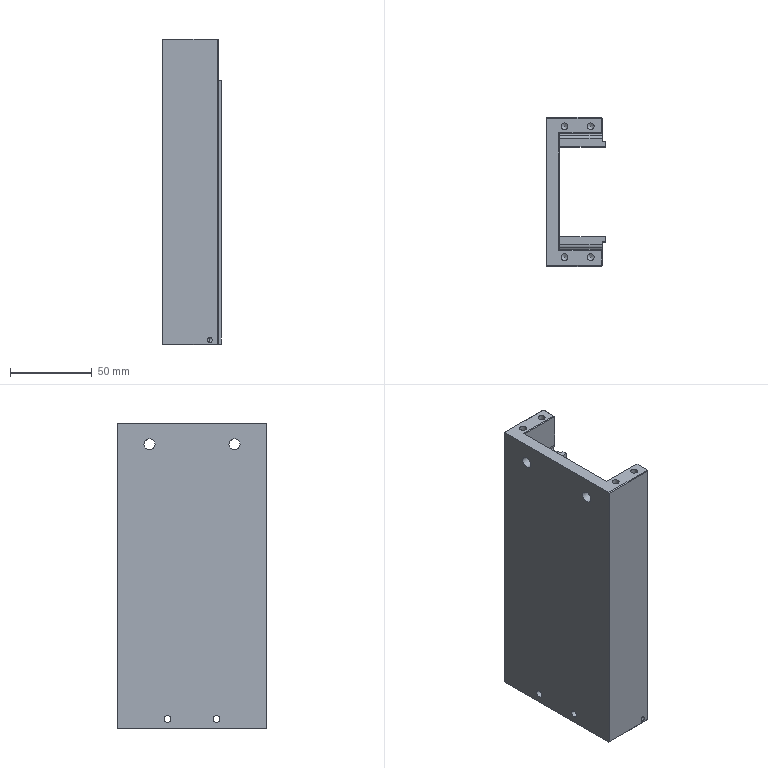CAM job | NX | 3+2 milling, drilling | part box 36 x 91 x 187 mm | stock box 40 x 100 x 192 mm
Tools:
number,name,description,diameter,corner_radius,flute_length,length,flutes
18,D2,平底铣刀-粗,2.0,0.0,50.0,75.0,2
9,D10,平底铣刀-粗,10.0,0.0,35.0,75.0,2
19,D2-J,平底铣刀-精,2.0,0.0,50.0,75.0,2
11,D3-J,平底铣刀-精,2.95,0.0,50.0,75.0,2
7,D6-J,平底铣刀-精,6.0,0.0,25.0,75.0,2
10,D10-J,平底铣刀-精,10.0,0.0,35.0,75.0,2
1,D80R0.8飞刀,圆鼻刀-粗,80.0,0.8,50.0,75.0,2
1,D80R0.8飞刀-J,圆鼻刀-精,80.0,0.8,50.0,75.0,2
2,D6倒角刀,倒角刀,6.0,0.0,3.0,25.0,2
20,M3X0.5,丝锥,2.5,0.0,35.0,50.0,2
22,M5X0.8,丝锥,4.2,0.0,35.0,50.0,2
23,M8X1.25,丝锥,6.8,0.0,35.0,50.0,2
12,ZT2.5,钻头,2.5,0.0,35.0,50.0,2
17,ZT2.8,钻头,2.8,0.0,35.0,50.0,2
16,ZT6.8,钻头,6.8,0.0,35.0,50.0,2
14,DRILL4.2,Twist Drill 4.2 mm,4.2,0.0,41.0,41.738,2
Operations:
program,operation,operation_type,tool,method,geometry_group,spindle_rpm,surface_speed,feed_per_tooth,feed_cut,feed_plunge,cut_length_mm,path_length_mm,cut_time_min,machine_time_min
B,FLOORMILL_FACEROUGH_COPY,VolumeBased25DMillingOperation,D80R0.8飞刀,LAYERROUGH-DEPTHK-STEPG,W-B,2800.0,703.696,0.5357,3000.0,100.0,4141.882,4389.788,1.381,1.405
B,FLOORMILL_FACEFINISH_COPY,VolumeBased25DMillingOperation,D80R0.8飞刀-J,SIDEFINISH-DEPTHK-STEPG,W-B,4000.0,1005.28,0.125,1000.0,100.0,591.11,627.11,0.5911,0.5947
B,FLOORMILL_LAYERROUGH-MID_COPY,VolumeBased25DMillingOperation,D10,LAYERROUGH-DEPTHK-STEPG,W-B,8000.0,251.327,0.3125,5000.0,100.0,82399.709,83354.509,16.48,16.575
B,FLOORMILL_LAYERROUGH-MID_COPY_COPY,VolumeBased25DMillingOperation,D10,LAYERROUGH-DEPTHK-STEPG,W-B,8000.0,251.327,0.3125,5000.0,100.0,6746.96,6888.849,1.349,1.364
B,SPOTDRILL-DEPTH0.8_2,Operation,D6倒角刀,NONE,W-B,8000.0,150.796,0.0312,500.0,90.0,21.6,685.36,0.0432,0.1096
B,BLINDCONE-M3TAPDRILL,Operation,ZT2.5,NONE,W-B,3000.0,23.562,0.0167,100.0,90.0,104.0,575.082,1.04,1.087
B,BLINDHOLE-FINISH3.0PILOT,Operation,ZT2.8,NONE,W-B,3000.0,26.389,0.0133,80.0,90.0,67.541,504.265,0.8443,0.8879
B,HOLEMILL_ROUGH_D2_1,CylinderMilling,D2,NONE,W-B,8000.0,50.266,0.0375,600.0,100.0,160.744,333.744,0.2679,0.2852
B,ZLEVEL_SMOOTH_D6REF12_COPY,ZLevelMilling,D3-J,LAYERFINISH-DEPTHK-STEPG,W-B,8000.0,74.142,0.0938,1500.0,100.0,3996.329,4160.168,2.664,2.681
B,DRILLCHAMFER_1,Operation,D6倒角刀,METHOD,W-B,8000.0,150.796,0.0312,500.0,0.0,38.0,457.733,0.076,0.118
B,DRILLCHAMFER_2,Operation,D6倒角刀,METHOD,W-B,8000.0,150.796,0.0312,500.0,0.0,9.6,142.259,0.0192,0.0325
B,DRILLCHAMFER_3,Operation,D6倒角刀,METHOD,W-B,8000.0,150.796,0.0625,1000.0,0.0,11.4,151.95,0.0114,0.0255
B,MILLCHAMFER_3,PlanarMilling,D6倒角刀,METHOD,W-B,8000.0,150.796,0.0375,600.0,100.0,62.549,314.149,0.1042,0.1294
B,PLANARDEBURR6X45L_COPY,SurfaceContour,D6倒角刀,CLIMBCHAMFER-DEPTH0-STEPG,W-B,6500.0,122.519,0.1154,1500.0,100.0,867.472,1812.47,0.5783,0.6728
B,PLANARDEBURR6X45L_COPY_1,SurfaceContour,D6倒角刀,CLIMBCHAMFER-DEPTH0-STEPG,W-B,6500.0,122.519,0.1154,1500.0,100.0,547.234,712.232,0.3648,0.3813
B,FLOORMILL_CHAMFER_COPY,VolumeBased25DMillingOperation,D6倒角刀,CLIMBCHAMFER-DEPTH0-STEPG,W-B,6500.0,122.519,0.1154,1500.0,100.0,30.37,156.355,0.0202,0.0328
B,HOLEMILL_FINISH_D2_1,CylinderMilling,D2-J,FINISHSTEPDEPTHOFF,W-B,8000.0,50.266,0.0125,200.0,100.0,46.2,219.201,0.231,0.2483
B,BLINDCONE-TAPM3,Operation,M3X0.5,METHOD,W-B,1000.0,7.854,0.0003,0.5,90.0,72.0,511.082,144.0,144.044
B,FLOORMILL_FINISHBOTTOM-MID_COPY,VolumeBased25DMillingOperation,D6-J,FINISHSTEPDEPTHOFF,W-B,7000.0,175.0,0.0536,1500.0,100.0,1953.022,2067.921,1.302,1.313
B,FLOORMILL_FINISHBOTTOM-MID_COPY_1,VolumeBased25DMillingOperation,D6-J,FINISHSTEPDEPTHOFF,W-B,7000.0,175.0,0.0536,1500.0,100.0,3522.626,3602.626,2.348,2.356
B,FLOORMILL_FINISHSIDE-MID-SELBOTTOM_COPY,VolumeBased25DMillingOperation,D6-J,SIDEFINISH-DEPTHK-STEPG,W-B,8000.0,150.792,0.0625,1000.0,100.0,396.34,503.14,0.3963,0.407
B,FLOORMILL_FINISHSIDE-MID-SELBOTTOM_COPY_1,VolumeBased25DMillingOperation,D6-J,SIDEFINISH-DEPTHK-STEPG,W-B,8000.0,150.792,0.0625,1000.0,100.0,828.022,1066.958,0.828,0.8519
B,ZLEVEL_FINISH-MID_COPY,ZLevelMilling,D6-J,SIDEFINISH-DEPTHK-STEPG,W-B,8000.0,150.792,0.0625,1000.0,100.0,22.905,229.451,0.0229,0.0436
A,TOPFACE,FaceMilling,D80R0.8飞刀,SIDEFINISH-DEPTHK-STEPG,W-A,4000.0,1005.31,0.125,1000.0,100.0,900.5,936.5,0.9005,0.9041
A,PROFILE_ROUGH_2,VolumeBased25DMillingOperation,D10,METHOD,W-A,8000.0,251.327,0.3125,5000.0,80.0,27584.539,27658.839,5.517,5.524
A,SPOTDRILL-DEPTH0.8,Operation,D6倒角刀,NONE,W-A,8000.0,150.796,0.0312,500.0,90.0,7.2,307.789,0.0144,0.0445
A,THRUHOLE-M5TAPDRILL,Operation,DRILL4.2,NONE,W-A,3000.0,39.584,0.0583,350.0,90.0,32.524,136.064,0.0929,0.1033
A,THRUHOLE-M8TAPDRILL,Operation,ZT6.8,NONE,W-A,1800.0,38.453,0.0972,350.0,90.0,36.086,165.181,0.1031,0.116
A,SOLIDONLY,SurfaceContour,D6倒角刀,METHOD,W-A,8000.0,150.796,0.1875,3000.0,100.0,572.13,607.931,0.1907,0.1943
A,MILLCHAMFER_1,PlanarMilling,D6倒角刀,METHOD,W-A,8000.0,150.796,0.0312,500.0,100.0,36.041,146.653,0.0721,0.0831
A,MILLCHAMFER_2,PlanarMilling,D6倒角刀,METHOD,W-A,8000.0,150.796,0.0375,600.0,100.0,48.803,181.002,0.0813,0.0946
A,THRUHOLE-TAPM5,Operation,M5X0.8,METHOD,W-A,500.0,6.597,0.0008,0.8,90.0,25.0,121.017,31.25,31.26
A,THRUHOLE-TAPM8,Operation,M8X1.25,METHOD,W-A,500.0,10.681,0.0013,1.25,90.0,26.0,145.01,20.8,20.812
A,PROFILE_SEMI_2,VolumeBased25DMillingOperation,D10-J,METHOD,W-A,8000.0,251.327,0.0625,1000.0,100.0,1182.405,1370.32,1.182,1.201